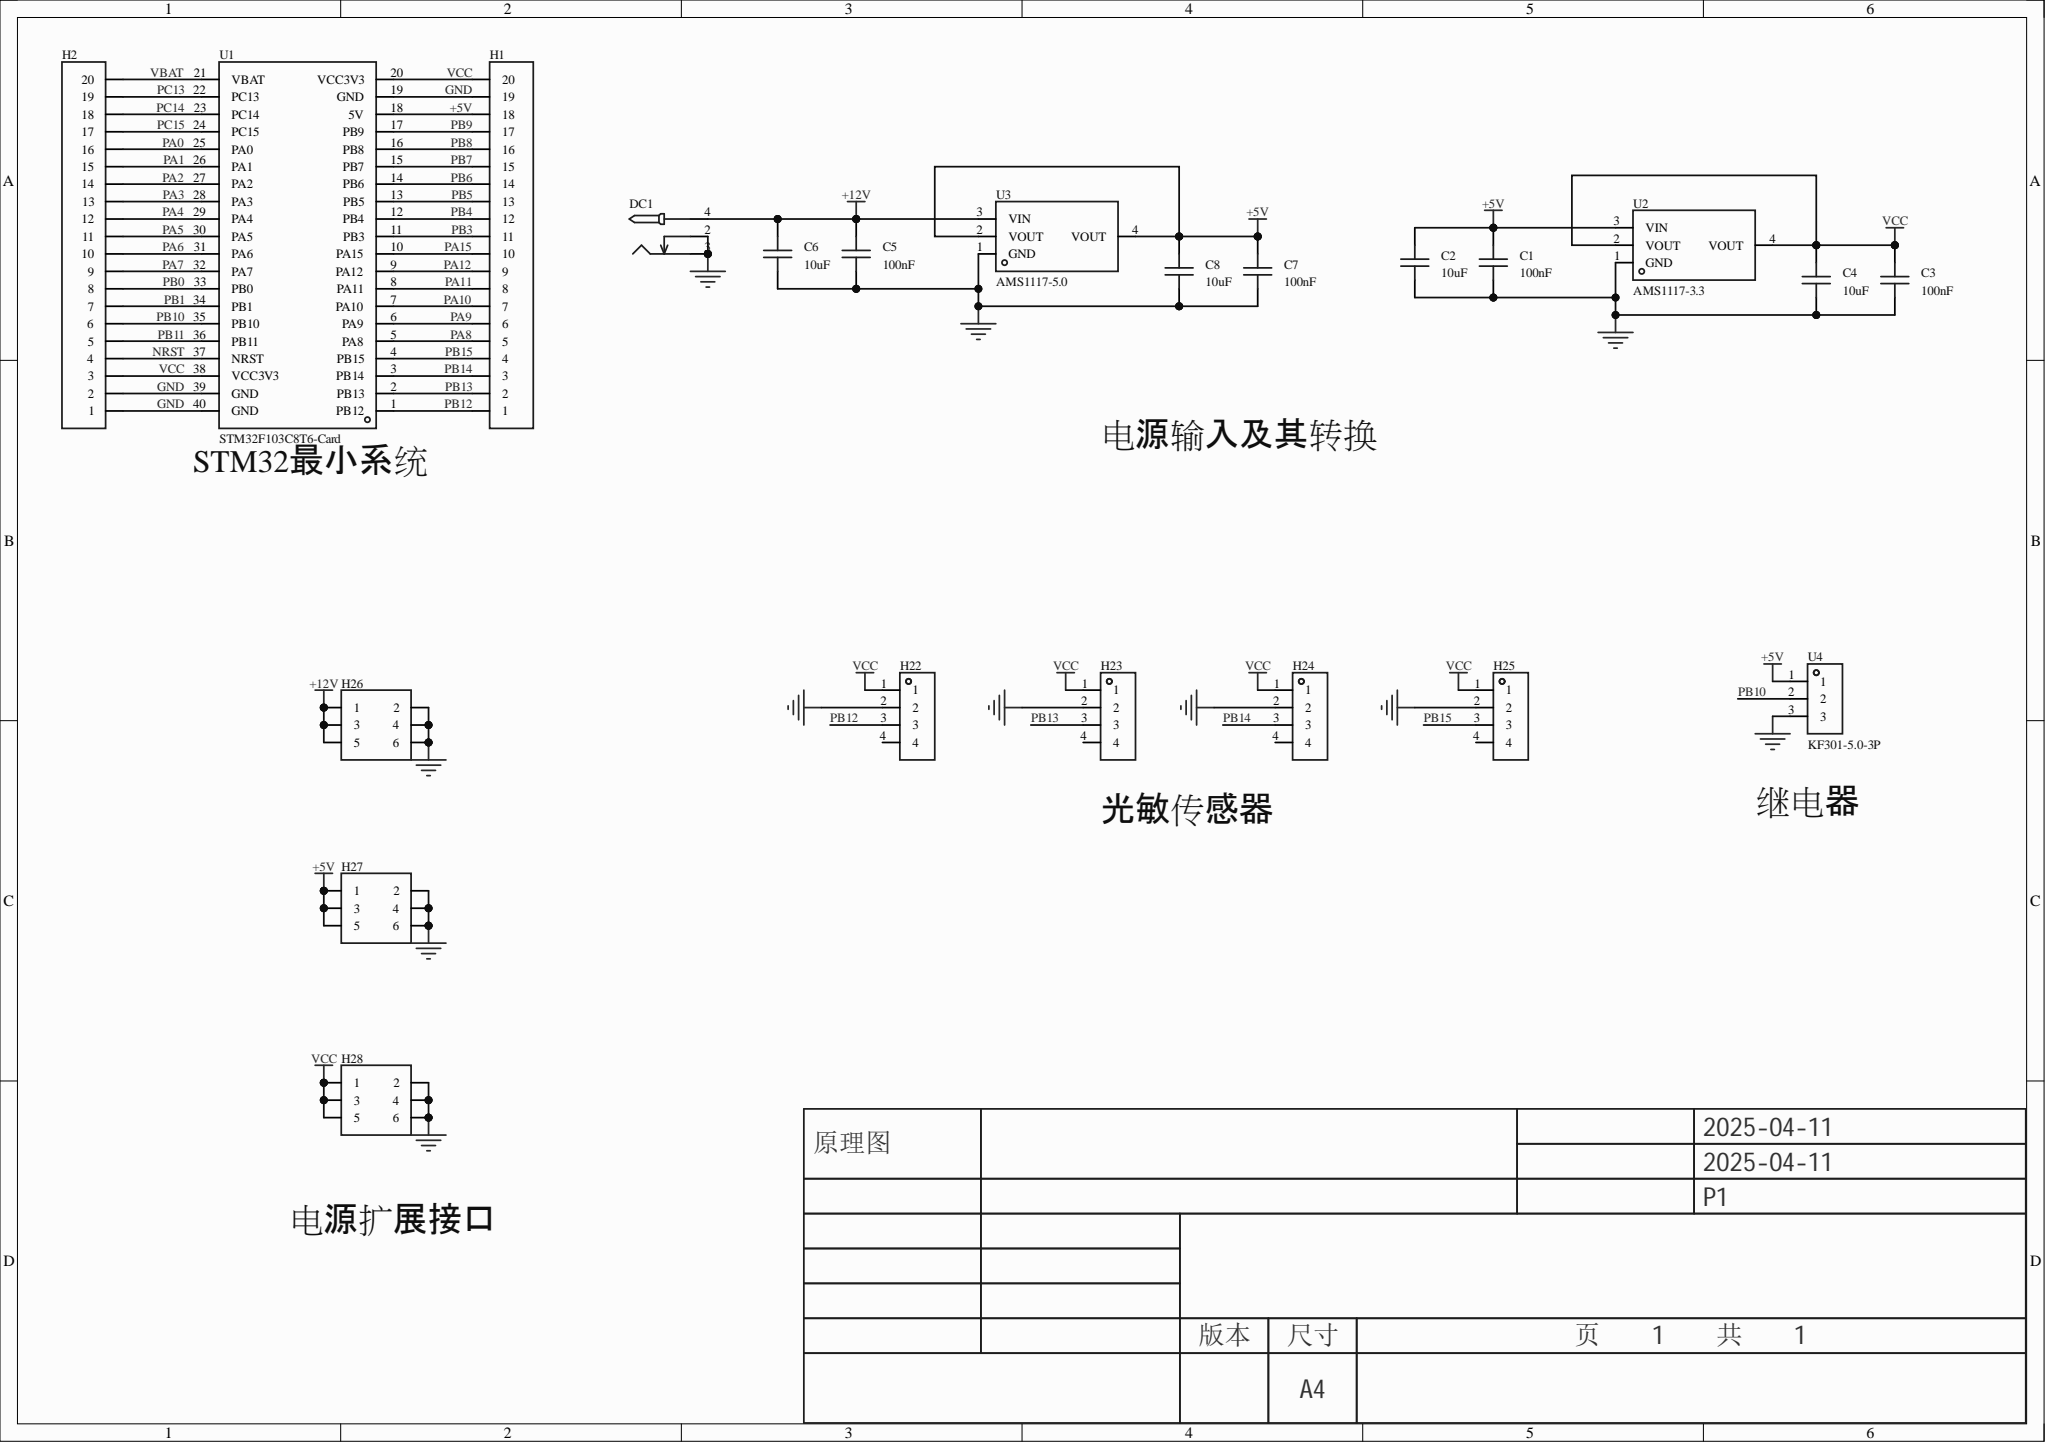Circuit board | Altium Designer | 22 parts | 38 nets
Bill of materials:
Comment,Description,Designator,Footprint,LibRef,Quantity
"100nF","","C1, C3, C5, C7","C0603","CAP_0603","4"
"10uF","","C2, C4, C6, C8","C0603","CAP_0603","4"
"","","DC1","DC-2.0","DC-005_2.0","1"
"","","H1, H2","HDR-TH_20P-P2.54-V-F","HDR-F_2.54_1x20P","2"
"","","H22, H23, H24, H25","HDR-TH_4P-P2.54-V-F","HDR-F_2.54_1x4P","4"
"","","H26, H27, H28","HDR-TH_6P-P2.54-V-F-R2-C3-S2.54","HDR-F_2.54_2x3","3"
"STM32F103C8T6-Card","","U1","CONN-TH_L53.3-W22.9_STM32F103C8T6-CARD","STM32F103C8T6-Card","1"
"AMS1117-3.3","输出类型:固定;工作电压:-;输出电压:3.3V;输出电流:1A;电源纹波抑制比(PSRR):72dB@(120Hz);输出极性:正极;","U2","SOT-223-3_L6.5-W3.4-P2.30-LS7.0-BR","AMS1117-3.3_C6186","1"
"AMS1117-5.0","输出类型:固定;工作电压:-;输出电压:3.3V;输出电流:1A;电源纹波抑制比(PSRR):72dB@(120Hz);输出极性:正极;","U3","SOT-223-3_L6.5-W3.4-P2.30-LS7.0-BR","AMS1117-3.3_C6186","1"
"KF301-5.0-3P","结构:1x3P;间距:5mm;颜色:蓝色;安装方式:直插;额定电流:17A;额定电压:250V;排数:1;线规 - AWG:14~22;线规 - 平方毫米:1.5;每排PIN数:3;工作温度范围:-30℃~+120℃;","U4","CONN-TH_3P-P5.00_KF301-5.0-3P","KF301-5.0-3P","1"
Netlist (Protel format):
[
C1
C0603
100nF



]
[
C2
C0603
10uF



]
[
C3
C0603
100nF



]
[
C4
C0603
10uF



]
[
C5
C0603
100nF



]
[
C6
C0603
10uF



]
[
C7
C0603
100nF



]
[
C8
C0603
10uF



]
[
DC1
DC-2.0




]
[
H1
HDR-TH_20P-P2.54-V-F




]
[
H2
HDR-TH_20P-P2.54-V-F




]
[
H22
HDR-TH_4P-P2.54-V-F




]
[
H23
HDR-TH_4P-P2.54-V-F




]
[
H24
HDR-TH_4P-P2.54-V-F




]
[
H25
HDR-TH_4P-P2.54-V-F




]
[
H26
HDR-TH_6P-P2.54-V-F-R2-C3-S2.54




]
[
H27
HDR-TH_6P-P2.54-V-F-R2-C3-S2.54




]
[
H28
HDR-TH_6P-P2.54-V-F-R2-C3-S2.54




]
[
U1
CONN-TH_L53.3-W22.9_STM32F103C8T6-CARD
STM32F103C8T6-Card



]
[
U2
SOT-223-3_L6.5-W3.4-P2.30-LS7.0-BR
AMS1117-3.3



]
[
U3
SOT-223-3_L6.5-W3.4-P2.30-LS7.0-BR
AMS1117-5.0



]
[
U4
CONN-TH_3P-P5.00_KF301-5.0-3P
KF301-5.0-3P



]
(
VCC
C3-2
C4-2
H1-20
H2-3
H22-1
H23-1
H24-1
H25-1
H28-1
H28-3
H28-5
U1-20
U1-38
U2-2
U2-4
)
(
VBAT
H2-20
U1-21
)
(
PC15
H2-17
U1-24
)
(
PC14
H2-18
U1-23
)
(
PC13
H2-19
U1-22
)
(
PB15
H1-4
H25-3
U1-4
)
(
PB14
H1-3
H24-3
U1-3
)
(
PB13
H1-2
H23-3
U1-2
)
(
PB12
H1-1
H22-3
U1-1
)
(
PB11
H2-5
U1-36
)
(
PB10
H2-6
U1-35
U4-2
)
(
PB9
H1-17
U1-17
)
(
PB8
H1-16
U1-16
)
(
PB7
H1-15
U1-15
)
(
PB6
H1-14
U1-14
)
(
PB5
H1-13
U1-13
)
(
PB4
H1-12
U1-12
)
(
PB3
H1-11
U1-11
)
(
PB1
H2-7
U1-34
)
(
PB0
H2-8
U1-33
)
(
PA15
H1-10
U1-10
)
(
PA12
H1-9
U1-9
)
(
PA11
H1-8
U1-8
)
(
PA10
H1-7
U1-7
)
(
PA9
H1-6
U1-6
)
(
PA8
H1-5
U1-5
)
(
PA7
H2-9
U1-32
)
(
PA6
H2-10
U1-31
)
(
PA5
H2-11
U1-30
)
(
PA4
H2-12
U1-29
)
(
PA3
H2-13
U1-28
)
(
PA2
H2-14
U1-27
)
(
PA1
H2-15
U1-26
)
(
PA0
H2-16
U1-25
)
(
NRST
H2-4
U1-37
)
(
GND
C1-1
C2-1
C3-1
C4-1
C5-1
C6-1
C7-1
C8-1
DC1-2
DC1-3
H1-19
H2-1
H2-2
H22-2
H23-2
H24-2
H25-2
H26-2
H26-4
H26-6
H27-2
H27-4
H27-6
H28-2
H28-4
H28-6
U1-19
U1-39
U1-40
U2-1
U3-1
U4-3
)
(
+12V
C5-2
C6-2
DC1-4
H26-1
H26-3
H26-5
U3-3
)
(
+5V
C1-2
C2-2
C7-2
C8-2
H1-18
H27-1
H27-3
H27-5
U1-18
U2-3
U3-2
U3-4
U4-1
)